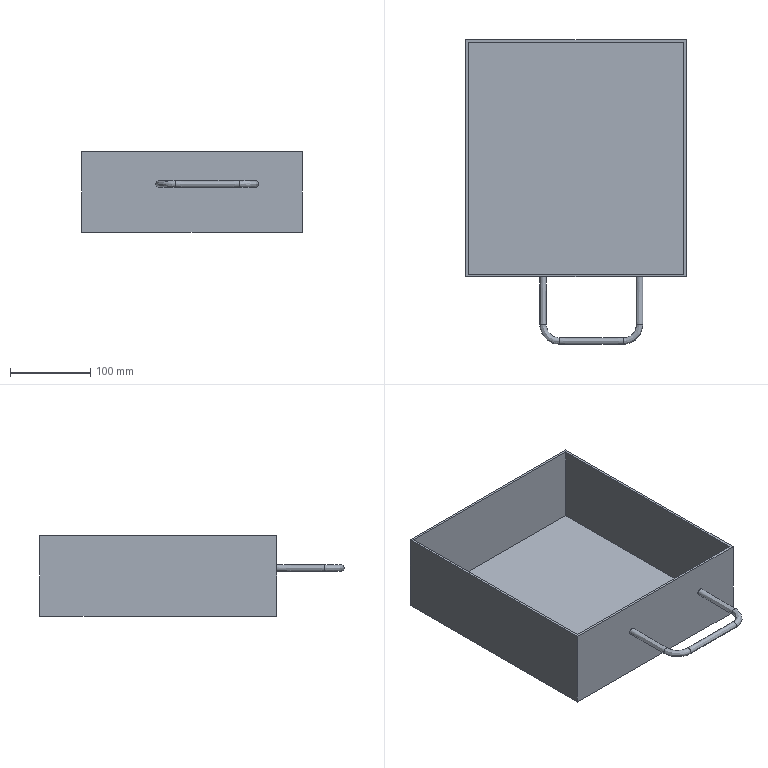Part | NX | features solid 2 | 1 solid | 16 faces | box 274 x 379 x 100 mm | volume 583374 mm3 | plane 11 | spline 5